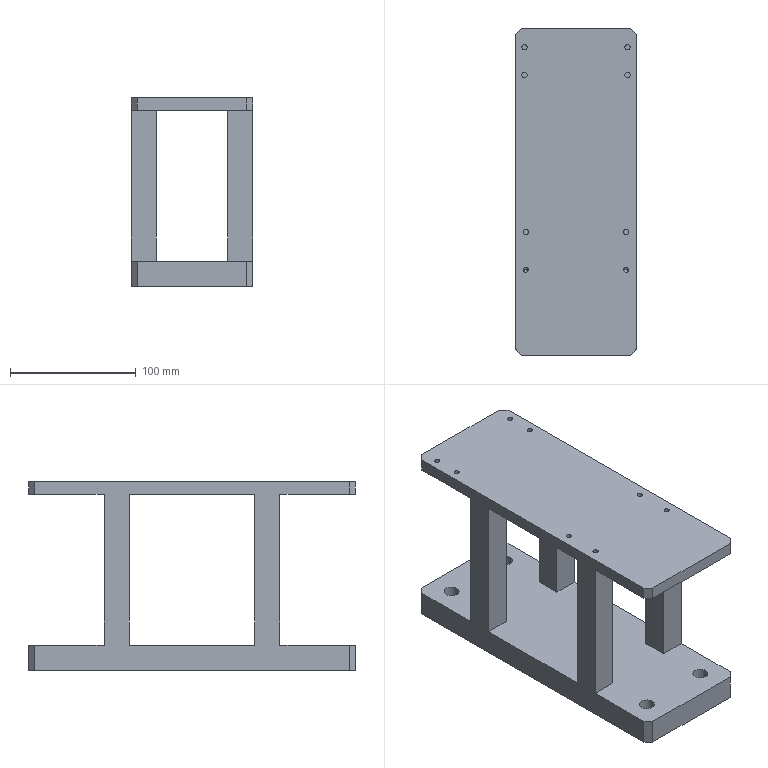Part | STEP file | Motor bracket | 1 solid | 58 faces | box 97 x 260 x 150 mm | volume 936866 mm3 | plane 30 | cylinder 24 | cone 4 | commonest cylinder face diameters 4.2 x16 12 x8